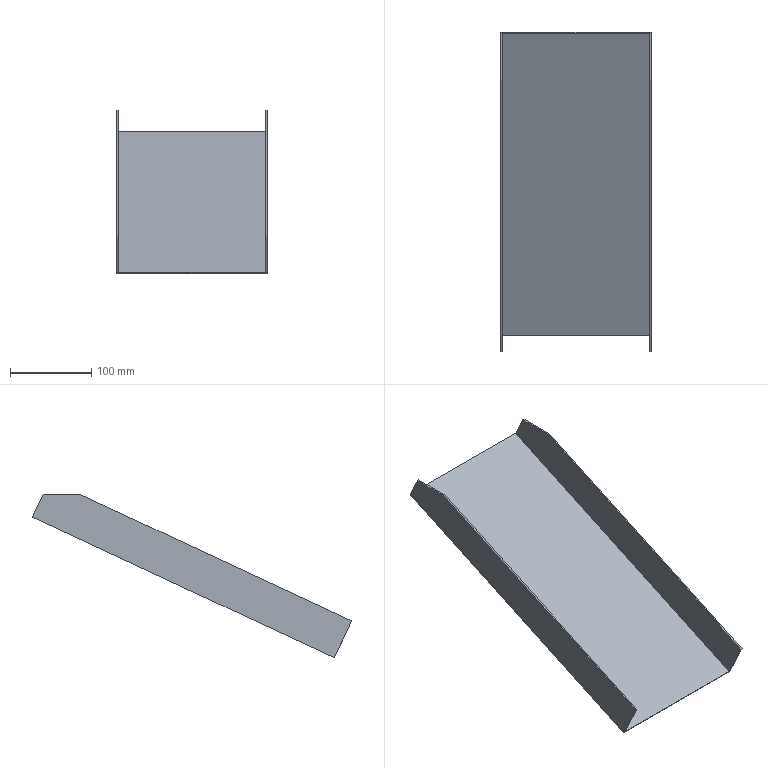Part | NX | features solid 2 | 1 solid | 12 faces | box 184.741 x 391.525 x 200.813 mm | volume 227920 mm3 | plane 12
STEP:
#1=CARTESIAN_POINT('',(-92.37,-229.606,-18.095));
#2=VERTEX_POINT('',#1);
#3=CARTESIAN_POINT('',(-92.37,-242.707,10.));
#4=VERTEX_POINT('',#3);
#5=CARTESIAN_POINT('',(-92.37,-229.606,-18.095));
#6=DIRECTION('',(0.,-0.4226,0.9063));
#7=VECTOR('',#6,1000.);
#8=LINE('',#5,#7);
#9=EDGE_CURVE('',#2,#4,#8,.T.);
#10=ORIENTED_EDGE('',*,*,#9,.T.);
#11=CARTESIAN_POINT('',(-90.37,-242.707,10.));
#12=VERTEX_POINT('',#11);
#13=CARTESIAN_POINT('',(17.63,-242.707,10.));
#14=DIRECTION('',(-1.,0.,0.));
#15=VECTOR('',#14,1000.);
#16=LINE('',#13,#15);
#17=EDGE_CURVE('',#4,#12,#16,.F.);
#18=ORIENTED_EDGE('',*,*,#17,.T.);
#19=CARTESIAN_POINT('',(-90.37,-230.452,-16.283));
#20=VERTEX_POINT('',#19);
#21=CARTESIAN_POINT('',(-90.37,-250.737,27.22));
#22=DIRECTION('',(0.,0.4226,-0.9063));
#23=VECTOR('',#22,1000.);
#24=LINE('',#21,#23);
#25=EDGE_CURVE('',#12,#20,#24,.T.);
#26=ORIENTED_EDGE('',*,*,#25,.T.);
#27=CARTESIAN_POINT('',(90.37,-230.452,-16.283));
#28=VERTEX_POINT('',#27);
#29=CARTESIAN_POINT('',(17.63,-230.452,-16.283));
#30=DIRECTION('',(1.,0.,0.));
#31=VECTOR('',#30,1000.);
#32=LINE('',#29,#31);
#33=EDGE_CURVE('',#28,#20,#32,.F.);
#34=ORIENTED_EDGE('',*,*,#33,.F.);
#35=CARTESIAN_POINT('',(90.37,-242.707,10.));
#36=VERTEX_POINT('',#35);
#37=CARTESIAN_POINT('',(90.37,-250.737,27.22));
#38=DIRECTION('',(0.,0.4226,-0.9063));
#39=VECTOR('',#38,1000.);
#40=LINE('',#37,#39);
#41=EDGE_CURVE('',#36,#28,#40,.T.);
#42=ORIENTED_EDGE('',*,*,#41,.F.);
#43=CARTESIAN_POINT('',(92.37,-242.707,10.));
#44=VERTEX_POINT('',#43);
#45=CARTESIAN_POINT('',(17.63,-242.707,10.));
#46=DIRECTION('',(-1.,0.,0.));
#47=VECTOR('',#46,1000.);
#48=LINE('',#45,#47);
#49=EDGE_CURVE('',#36,#44,#48,.F.);
#50=ORIENTED_EDGE('',*,*,#49,.T.);
#51=CARTESIAN_POINT('',(92.37,-229.606,-18.095));
#52=VERTEX_POINT('',#51);
#53=CARTESIAN_POINT('',(92.37,-229.606,-18.095));
#54=DIRECTION('',(0.,-0.4226,0.9063));
#55=VECTOR('',#54,1000.);
#56=LINE('',#53,#55);
#57=EDGE_CURVE('',#52,#44,#56,.T.);
#58=ORIENTED_EDGE('',*,*,#57,.F.);
#59=CARTESIAN_POINT('',(17.63,-229.606,-18.095));
#60=DIRECTION('',(1.,0.,0.));
#61=VECTOR('',#60,1000.);
#62=LINE('',#59,#61);
#63=EDGE_CURVE('',#52,#2,#62,.F.);
#64=ORIENTED_EDGE('',*,*,#63,.T.);
#65=EDGE_LOOP('',(#10,#18,#26,#34,#42,#50,#58,#64));
#66=FACE_BOUND('',#65,.T.);
#67=CARTESIAN_POINT('',(17.63,-229.606,-18.095));
#68=DIRECTION('',(0.,-0.9063,-0.4226));
#69=DIRECTION('',(-1.,0.,0.));
#70=AXIS2_PLACEMENT_3D('',#67,#68,#69);
#71=PLANE('',#70);
#72=ADVANCED_FACE('',(#66),#71,.F.);
#73=CARTESIAN_POINT('',(-92.37,-287.666,10.));
#74=VERTEX_POINT('',#73);
#75=CARTESIAN_POINT('',(-92.37,-621.131,-145.497));
#76=VERTEX_POINT('',#75);
#77=CARTESIAN_POINT('',(-92.37,-250.737,27.22));
#78=DIRECTION('',(0.,-0.9063,-0.4226));
#79=VECTOR('',#78,1000.);
#80=LINE('',#77,#79);
#81=EDGE_CURVE('',#74,#76,#80,.T.);
#82=ORIENTED_EDGE('',*,*,#81,.F.);
#83=CARTESIAN_POINT('',(-92.37,-265.859,10.));
#84=DIRECTION('',(0.,-1.,0.));
#85=VECTOR('',#84,1000.);
#86=LINE('',#83,#85);
#87=EDGE_CURVE('',#74,#4,#86,.F.);
#88=ORIENTED_EDGE('',*,*,#87,.T.);
#89=ORIENTED_EDGE('',*,*,#9,.F.);
#90=CARTESIAN_POINT('',(-92.37,-600.,-190.813));
#91=VERTEX_POINT('',#90);
#92=CARTESIAN_POINT('',(-92.37,-265.859,-35.));
#93=DIRECTION('',(0.,0.9063,0.4226));
#94=VECTOR('',#93,1000.);
#95=LINE('',#92,#94);
#96=EDGE_CURVE('',#2,#91,#95,.F.);
#97=ORIENTED_EDGE('',*,*,#96,.T.);
#98=CARTESIAN_POINT('',(-92.37,-621.131,-145.497));
#99=DIRECTION('',(0.,0.4226,-0.9063));
#100=VECTOR('',#99,1000.);
#101=LINE('',#98,#100);
#102=EDGE_CURVE('',#76,#91,#101,.T.);
#103=ORIENTED_EDGE('',*,*,#102,.F.);
#104=EDGE_LOOP('',(#82,#88,#89,#97,#103));
#105=FACE_BOUND('',#104,.T.);
#106=CARTESIAN_POINT('',(-92.37,-265.859,-35.));
#107=DIRECTION('',(1.,0.,0.));
#108=DIRECTION('',(0.,-0.9063,-0.4226));
#109=AXIS2_PLACEMENT_3D('',#106,#107,#108);
#110=PLANE('',#109);
#111=ADVANCED_FACE('',(#105),#110,.F.);
#112=CARTESIAN_POINT('',(-90.37,-287.666,10.));
#113=VERTEX_POINT('',#112);
#114=CARTESIAN_POINT('',(-90.37,-621.131,-145.497));
#115=VERTEX_POINT('',#114);
#116=CARTESIAN_POINT('',(-90.37,-250.737,27.22));
#117=DIRECTION('',(0.,-0.9063,-0.4226));
#118=VECTOR('',#117,1000.);
#119=LINE('',#116,#118);
#120=EDGE_CURVE('',#113,#115,#119,.T.);
#121=ORIENTED_EDGE('',*,*,#120,.F.);
#122=CARTESIAN_POINT('',(-92.37,-287.666,10.));
#123=DIRECTION('',(-1.,0.,0.));
#124=VECTOR('',#123,1000.);
#125=LINE('',#122,#124);
#126=EDGE_CURVE('',#113,#74,#125,.T.);
#127=ORIENTED_EDGE('',*,*,#126,.T.);
#128=ORIENTED_EDGE('',*,*,#81,.T.);
#129=CARTESIAN_POINT('',(-92.37,-621.131,-145.497));
#130=DIRECTION('',(1.,0.,0.));
#131=VECTOR('',#130,1000.);
#132=LINE('',#129,#131);
#133=EDGE_CURVE('',#76,#115,#132,.T.);
#134=ORIENTED_EDGE('',*,*,#133,.T.);
#135=EDGE_LOOP('',(#121,#127,#128,#134));
#136=FACE_BOUND('',#135,.T.);
#137=CARTESIAN_POINT('',(-92.37,-250.737,27.22));
#138=DIRECTION('',(0.,-0.4226,0.9063));
#139=DIRECTION('',(0.,-0.9063,-0.4226));
#140=AXIS2_PLACEMENT_3D('',#137,#138,#139);
#141=PLANE('',#140);
#142=ADVANCED_FACE('',(#136),#141,.T.);
#143=ORIENTED_EDGE('',*,*,#25,.F.);
#144=CARTESIAN_POINT('',(-90.37,-250.737,10.));
#145=DIRECTION('',(0.,-1.,0.));
#146=VECTOR('',#145,1000.);
#147=LINE('',#144,#146);
#148=EDGE_CURVE('',#12,#113,#147,.T.);
#149=ORIENTED_EDGE('',*,*,#148,.T.);
#150=ORIENTED_EDGE('',*,*,#120,.T.);
#151=CARTESIAN_POINT('',(-90.37,-600.845,-189.));
#152=VERTEX_POINT('',#151);
#153=CARTESIAN_POINT('',(-90.37,-621.131,-145.497));
#154=DIRECTION('',(0.,0.4226,-0.9063));
#155=VECTOR('',#154,1000.);
#156=LINE('',#153,#155);
#157=EDGE_CURVE('',#115,#152,#156,.T.);
#158=ORIENTED_EDGE('',*,*,#157,.T.);
#159=CARTESIAN_POINT('',(-90.37,-266.704,-33.187));
#160=DIRECTION('',(0.,-0.9063,-0.4226));
#161=VECTOR('',#160,1000.);
#162=LINE('',#159,#161);
#163=EDGE_CURVE('',#20,#152,#162,.T.);
#164=ORIENTED_EDGE('',*,*,#163,.F.);
#165=EDGE_LOOP('',(#143,#149,#150,#158,#164));
#166=FACE_BOUND('',#165,.T.);
#167=CARTESIAN_POINT('',(-90.37,-250.737,27.22));
#168=DIRECTION('',(1.,0.,0.));
#169=DIRECTION('',(0.,1.,0.));
#170=AXIS2_PLACEMENT_3D('',#167,#168,#169);
#171=PLANE('',#170);
#172=ADVANCED_FACE('',(#166),#171,.T.);
#173=ORIENTED_EDGE('',*,*,#57,.T.);
#174=CARTESIAN_POINT('',(92.37,-287.666,10.));
#175=VERTEX_POINT('',#174);
#176=CARTESIAN_POINT('',(92.37,-265.859,10.));
#177=DIRECTION('',(0.,1.,0.));
#178=VECTOR('',#177,1000.);
#179=LINE('',#176,#178);
#180=EDGE_CURVE('',#44,#175,#179,.F.);
#181=ORIENTED_EDGE('',*,*,#180,.T.);
#182=CARTESIAN_POINT('',(92.37,-621.131,-145.497));
#183=VERTEX_POINT('',#182);
#184=CARTESIAN_POINT('',(92.37,-250.737,27.22));
#185=DIRECTION('',(0.,-0.9063,-0.4226));
#186=VECTOR('',#185,1000.);
#187=LINE('',#184,#186);
#188=EDGE_CURVE('',#175,#183,#187,.T.);
#189=ORIENTED_EDGE('',*,*,#188,.T.);
#190=CARTESIAN_POINT('',(92.37,-600.,-190.813));
#191=VERTEX_POINT('',#190);
#192=CARTESIAN_POINT('',(92.37,-621.131,-145.497));
#193=DIRECTION('',(0.,0.4226,-0.9063));
#194=VECTOR('',#193,1000.);
#195=LINE('',#192,#194);
#196=EDGE_CURVE('',#183,#191,#195,.T.);
#197=ORIENTED_EDGE('',*,*,#196,.T.);
#198=CARTESIAN_POINT('',(92.37,-265.859,-35.));
#199=DIRECTION('',(0.,0.9063,0.4226));
#200=VECTOR('',#199,1000.);
#201=LINE('',#198,#200);
#202=EDGE_CURVE('',#52,#191,#201,.F.);
#203=ORIENTED_EDGE('',*,*,#202,.F.);
#204=EDGE_LOOP('',(#173,#181,#189,#197,#203));
#205=FACE_BOUND('',#204,.T.);
#206=CARTESIAN_POINT('',(92.37,-265.859,-35.));
#207=DIRECTION('',(-1.,0.,0.));
#208=DIRECTION('',(0.,-0.9063,-0.4226));
#209=AXIS2_PLACEMENT_3D('',#206,#207,#208);
#210=PLANE('',#209);
#211=ADVANCED_FACE('',(#205),#210,.F.);
#212=ORIENTED_EDGE('',*,*,#188,.F.);
#213=CARTESIAN_POINT('',(90.37,-287.666,10.));
#214=VERTEX_POINT('',#213);
#215=CARTESIAN_POINT('',(92.37,-287.666,10.));
#216=DIRECTION('',(-1.,0.,0.));
#217=VECTOR('',#216,1000.);
#218=LINE('',#215,#217);
#219=EDGE_CURVE('',#175,#214,#218,.T.);
#220=ORIENTED_EDGE('',*,*,#219,.T.);
#221=CARTESIAN_POINT('',(90.37,-621.131,-145.497));
#222=VERTEX_POINT('',#221);
#223=CARTESIAN_POINT('',(90.37,-250.737,27.22));
#224=DIRECTION('',(0.,-0.9063,-0.4226));
#225=VECTOR('',#224,1000.);
#226=LINE('',#223,#225);
#227=EDGE_CURVE('',#214,#222,#226,.T.);
#228=ORIENTED_EDGE('',*,*,#227,.T.);
#229=CARTESIAN_POINT('',(92.37,-621.131,-145.497));
#230=DIRECTION('',(-1.,0.,0.));
#231=VECTOR('',#230,1000.);
#232=LINE('',#229,#231);
#233=EDGE_CURVE('',#183,#222,#232,.T.);
#234=ORIENTED_EDGE('',*,*,#233,.F.);
#235=EDGE_LOOP('',(#212,#220,#228,#234));
#236=FACE_BOUND('',#235,.T.);
#237=CARTESIAN_POINT('',(92.37,-250.737,27.22));
#238=DIRECTION('',(0.,-0.4226,0.9063));
#239=DIRECTION('',(0.,-0.9063,-0.4226));
#240=AXIS2_PLACEMENT_3D('',#237,#238,#239);
#241=PLANE('',#240);
#242=ADVANCED_FACE('',(#236),#241,.T.);
#243=ORIENTED_EDGE('',*,*,#227,.F.);
#244=CARTESIAN_POINT('',(90.37,-250.737,10.));
#245=DIRECTION('',(0.,1.,0.));
#246=VECTOR('',#245,1000.);
#247=LINE('',#244,#246);
#248=EDGE_CURVE('',#214,#36,#247,.T.);
#249=ORIENTED_EDGE('',*,*,#248,.T.);
#250=ORIENTED_EDGE('',*,*,#41,.T.);
#251=CARTESIAN_POINT('',(90.37,-600.845,-189.));
#252=VERTEX_POINT('',#251);
#253=CARTESIAN_POINT('',(90.37,-266.704,-33.187));
#254=DIRECTION('',(0.,-0.9063,-0.4226));
#255=VECTOR('',#254,1000.);
#256=LINE('',#253,#255);
#257=EDGE_CURVE('',#28,#252,#256,.T.);
#258=ORIENTED_EDGE('',*,*,#257,.T.);
#259=CARTESIAN_POINT('',(90.37,-621.131,-145.497));
#260=DIRECTION('',(0.,0.4226,-0.9063));
#261=VECTOR('',#260,1000.);
#262=LINE('',#259,#261);
#263=EDGE_CURVE('',#222,#252,#262,.T.);
#264=ORIENTED_EDGE('',*,*,#263,.F.);
#265=EDGE_LOOP('',(#243,#249,#250,#258,#264));
#266=FACE_BOUND('',#265,.T.);
#267=CARTESIAN_POINT('',(90.37,-250.737,27.22));
#268=DIRECTION('',(-1.,0.,0.));
#269=DIRECTION('',(0.,1.,0.));
#270=AXIS2_PLACEMENT_3D('',#267,#268,#269);
#271=PLANE('',#270);
#272=ADVANCED_FACE('',(#266),#271,.T.);
#273=CARTESIAN_POINT('',(17.63,-600.,-190.813));
#274=DIRECTION('',(-1.,0.,0.));
#275=VECTOR('',#274,1000.);
#276=LINE('',#273,#275);
#277=EDGE_CURVE('',#191,#91,#276,.T.);
#278=ORIENTED_EDGE('',*,*,#277,.F.);
#279=ORIENTED_EDGE('',*,*,#196,.F.);
#280=ORIENTED_EDGE('',*,*,#233,.T.);
#281=ORIENTED_EDGE('',*,*,#263,.T.);
#282=CARTESIAN_POINT('',(17.63,-600.845,-189.));
#283=DIRECTION('',(-1.,0.,0.));
#284=VECTOR('',#283,1000.);
#285=LINE('',#282,#284);
#286=EDGE_CURVE('',#252,#152,#285,.T.);
#287=ORIENTED_EDGE('',*,*,#286,.T.);
#288=ORIENTED_EDGE('',*,*,#157,.F.);
#289=ORIENTED_EDGE('',*,*,#133,.F.);
#290=ORIENTED_EDGE('',*,*,#102,.T.);
#291=EDGE_LOOP('',(#278,#279,#280,#281,#287,#288,#289,#290));
#292=FACE_BOUND('',#291,.T.);
#293=CARTESIAN_POINT('',(-92.37,-621.131,-145.497));
#294=DIRECTION('',(0.,-0.9063,-0.4226));
#295=DIRECTION('',(0.,0.4226,-0.9063));
#296=AXIS2_PLACEMENT_3D('',#293,#294,#295);
#297=PLANE('',#296);
#298=ADVANCED_FACE('',(#292),#297,.T.);
#299=ORIENTED_EDGE('',*,*,#286,.F.);
#300=ORIENTED_EDGE('',*,*,#257,.F.);
#301=ORIENTED_EDGE('',*,*,#33,.T.);
#302=ORIENTED_EDGE('',*,*,#163,.T.);
#303=EDGE_LOOP('',(#299,#300,#301,#302));
#304=FACE_BOUND('',#303,.T.);
#305=CARTESIAN_POINT('',(17.63,-266.704,-33.187));
#306=DIRECTION('',(0.,0.4226,-0.9063));
#307=DIRECTION('',(0.,0.9063,0.4226));
#308=AXIS2_PLACEMENT_3D('',#305,#306,#307);
#309=PLANE('',#308);
#310=ADVANCED_FACE('',(#304),#309,.F.);
#311=ORIENTED_EDGE('',*,*,#63,.F.);
#312=ORIENTED_EDGE('',*,*,#202,.T.);
#313=ORIENTED_EDGE('',*,*,#277,.T.);
#314=ORIENTED_EDGE('',*,*,#96,.F.);
#315=EDGE_LOOP('',(#311,#312,#313,#314));
#316=FACE_BOUND('',#315,.T.);
#317=CARTESIAN_POINT('',(17.63,-265.859,-35.));
#318=DIRECTION('',(0.,0.4226,-0.9063));
#319=DIRECTION('',(0.,0.9063,0.4226));
#320=AXIS2_PLACEMENT_3D('',#317,#318,#319);
#321=PLANE('',#320);
#322=ADVANCED_FACE('',(#316),#321,.T.);
#323=ORIENTED_EDGE('',*,*,#49,.F.);
#324=ORIENTED_EDGE('',*,*,#248,.F.);
#325=ORIENTED_EDGE('',*,*,#219,.F.);
#326=ORIENTED_EDGE('',*,*,#180,.F.);
#327=EDGE_LOOP('',(#323,#324,#325,#326));
#328=FACE_BOUND('',#327,.T.);
#329=CARTESIAN_POINT('',(35.,380.,10.));
#330=DIRECTION('',(0.,0.,1.));
#331=DIRECTION('',(1.,0.,0.));
#332=AXIS2_PLACEMENT_3D('',#329,#330,#331);
#333=PLANE('',#332);
#334=ADVANCED_FACE('',(#328),#333,.T.);
#335=ORIENTED_EDGE('',*,*,#17,.F.);
#336=ORIENTED_EDGE('',*,*,#87,.F.);
#337=ORIENTED_EDGE('',*,*,#126,.F.);
#338=ORIENTED_EDGE('',*,*,#148,.F.);
#339=EDGE_LOOP('',(#335,#336,#337,#338));
#340=FACE_BOUND('',#339,.T.);
#341=CARTESIAN_POINT('',(35.,380.,10.));
#342=DIRECTION('',(0.,0.,1.));
#343=DIRECTION('',(1.,0.,0.));
#344=AXIS2_PLACEMENT_3D('',#341,#342,#343);
#345=PLANE('',#344);
#346=ADVANCED_FACE('',(#340),#345,.T.);
#347=CLOSED_SHELL('',(#72,#111,#142,#172,#211,#242,#272,#298,#310,#322,#334,#346));
#348=MANIFOLD_SOLID_BREP('',#347);
#349=(LENGTH_UNIT()NAMED_UNIT(*)SI_UNIT(.MILLI.,.METRE.));
#350=UNCERTAINTY_MEASURE_WITH_UNIT(LENGTH_MEASURE(0.00001),#349,'','');
#351=(NAMED_UNIT(*)PLANE_ANGLE_UNIT()SI_UNIT($,.RADIAN.));
#352=(NAMED_UNIT(*)SI_UNIT($,.STERADIAN.)SOLID_ANGLE_UNIT());
#353=(GEOMETRIC_REPRESENTATION_CONTEXT(3)GLOBAL_UNCERTAINTY_ASSIGNED_CONTEXT((#350))GLOBAL_UNIT_ASSIGNED_CONTEXT((#349,#351,#352))REPRESENTATION_CONTEXT('',''));
#354=ADVANCED_BREP_SHAPE_REPRESENTATION('',(#348),#353);